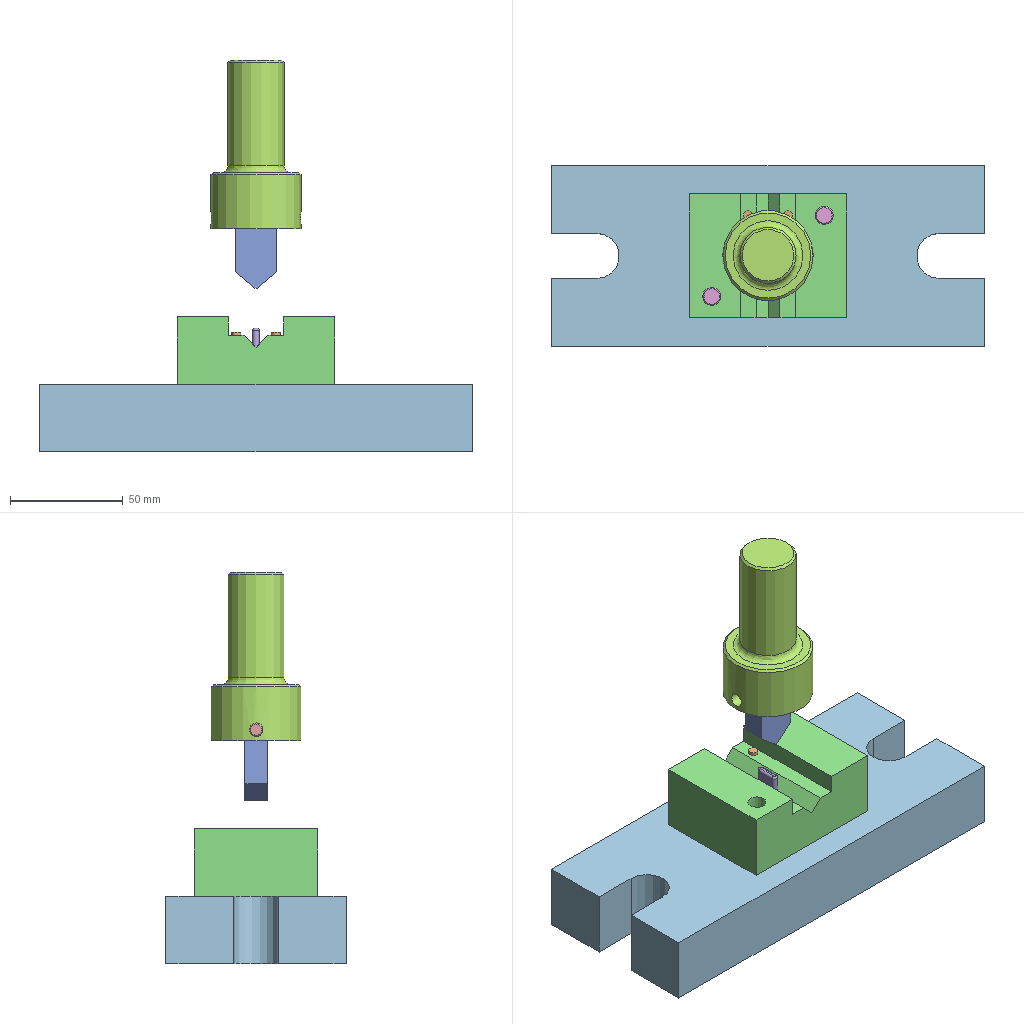Assembly | NX | 10 different items | 13 placed | box 192 x 80 x 174 mm
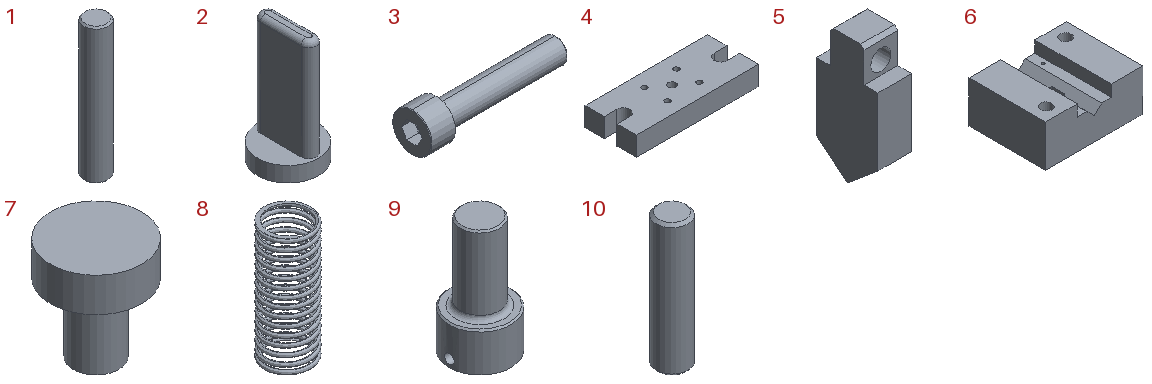Parts list (item | quantity | size | volume | features):
1 | x2 | 8 x 8 x 45 mm | 2256 mm3 | features DATUM_CSYS 2, CHAMFER 1, EXTRUDE 1, SKETCH 1
2 | x1 | 12 x 12 x 23 mm | 960.161 mm3 | features DATUM_CSYS 3, EXTRUDE 2, SKETCH 2, BLEND 1
3 | x2 | 48 x 13 x 13 mm | 2924 mm3 | features BREP 1
4 | x1 | 192 x 80 x 30 mm | 417369 mm3 | features DATUM_CSYS 5, EXTRUDE 4, SKETCH 4
5 | x1 | 10 x 18.2 x 37.6 mm | 5039 mm3 | features DATUM_CSYS 3, CHAMFER 2, EXTRUDE 2, SKETCH 2
6 | x1 | 70 x 55 x 30 mm | 96709 mm3 | features DATUM_CSYS 8, EXTRUDE 7, SKETCH 7, DATUM_PLANE 1
7 | x2 | 4 x 4 x 4.5 mm | 28.274 mm3 | features DATUM_CSYS 3, EXTRUDE 2, SKETCH 2
8 | x1 | - | 411.355 mm3 | features BREP 1
9 | x1 | 40 x 40 x 75 mm | 54175 mm3 | features DATUM_CSYS 5, EXTRUDE 4, SKETCH 4, CHAMFER 2, BLEND 1
10 | x1 | 6 x 6 x 25 mm | 702.408 mm3 | features CHAMFER 2, DATUM_CSYS 2, EXTRUDE 1, SKETCH 1
Mates (type | each side: item.copy, entity, surface, feature):
Fix | 4.1 component
Touch | 6.1 face cylinder Extrude(6) | 4.1 face cylinder Extrude(1) | 2 times
Touch | 2.1 face plane Extrude(1) | 6.1 face plane Extrude(4)
Touch | 6.1 face plane Extrude(1) | 4.1 face plane Extrude(1)
Touch | 7.1 face plane Extrude(2) | 6.1 face plane Extrude(5) | 2 times
Touch | 7.1 face cylinder Extrude(1) | 6.1 face cylinder Extrude(8) | 2 times
Touch | 3.1 face cylinder Body(1) | 6.1 face cylinder Extrude(7)
Touch | 3.1 face plane Body(1) | 4.1 face plane Extrude(2) | 2 times
Touch | 3.1 face cylinder Body(1) | 4.1 face cylinder Extrude(1)
Touch | 1.1 face cylinder Extrude(1) | 4.1 face cylinder Extrude(1) | 2 times
Touch | 1.1 face plane Extrude(1) | 4.1 face plane Extrude(1) | 2 times
Touch | 9.1 face cylinder Extrude(5) | 4.1 face cylinder Extrude(3)
Touch | 5.1 face cylinder Extrude(4) | 9.1 face cylinder Extrude(4)
Touch | 5.1 face plane Extrude(1) | 9.1 face plane Extrude(3)
Touch | 10.1 face cylinder Extrude(1) | 9.1 face cylinder Extrude(4)